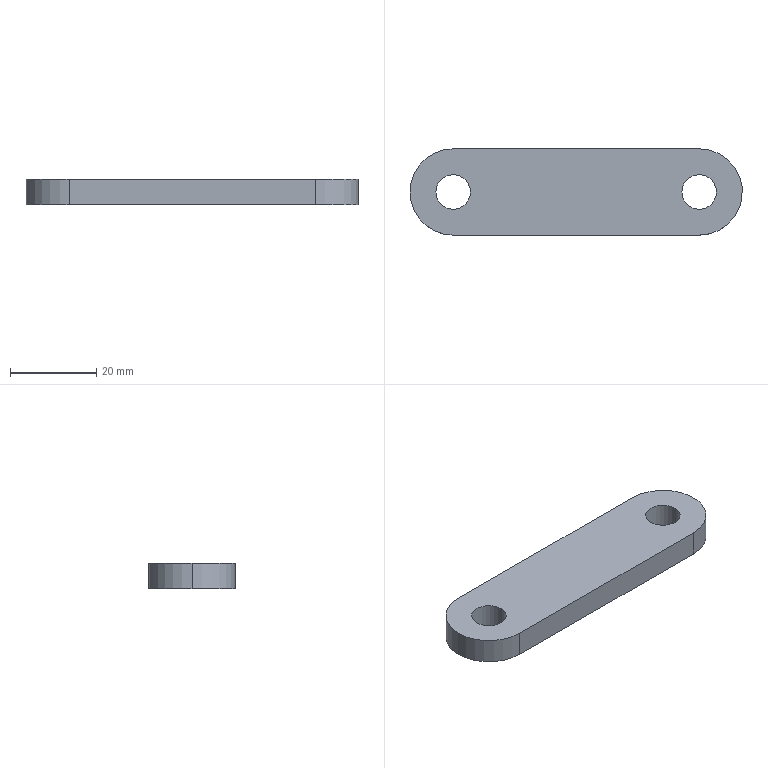Part | SolidWorks | features Extrusion 1, ICE 1 | 1 solid | 11 faces | box 77.02 x 20 x 6 mm | volume 8124 mm3 | cylinder 7 | plane 4 | commonest cylinder face diameters 8 x4 20 x3
STEP:
#1=CARTESIAN_POINT('',(53.02,0.,0.));
#2=VERTEX_POINT('',#1);
#3=CARTESIAN_POINT('',(61.02,0.,0.));
#4=VERTEX_POINT('',#3);
#5=CARTESIAN_POINT('',(57.02,0.,0.));
#6=DIRECTION('',(0.,0.,1.));
#7=DIRECTION('',(1.,0.,0.));
#8=AXIS2_PLACEMENT_3D('',#5,#6,#7);
#9=CIRCLE('',#8,4.);
#10=EDGE_CURVE('',#2,#4,#9,.T.);
#11=ORIENTED_EDGE('',*,*,#10,.F.);
#12=CARTESIAN_POINT('',(53.02,0.,6.));
#13=VERTEX_POINT('',#12);
#14=CARTESIAN_POINT('',(53.02,0.,-89.));
#15=DIRECTION('',(0.,0.,1.));
#16=VECTOR('',#15,1000.);
#17=LINE('',#14,#16);
#18=EDGE_CURVE('',#2,#13,#17,.T.);
#19=ORIENTED_EDGE('',*,*,#18,.T.);
#20=CARTESIAN_POINT('',(61.02,0.,6.));
#21=VERTEX_POINT('',#20);
#22=CARTESIAN_POINT('',(57.02,0.,6.));
#23=DIRECTION('',(0.,0.,1.));
#24=DIRECTION('',(1.,0.,0.));
#25=AXIS2_PLACEMENT_3D('',#22,#23,#24);
#26=CIRCLE('',#25,4.);
#27=EDGE_CURVE('',#13,#21,#26,.T.);
#28=ORIENTED_EDGE('',*,*,#27,.T.);
#29=CARTESIAN_POINT('',(61.02,0.,-89.));
#30=DIRECTION('',(0.,0.,1.));
#31=VECTOR('',#30,1000.);
#32=LINE('',#29,#31);
#33=EDGE_CURVE('',#4,#21,#32,.T.);
#34=ORIENTED_EDGE('',*,*,#33,.F.);
#35=EDGE_LOOP('',(#11,#19,#28,#34));
#36=FACE_OUTER_BOUND('',#35,.T.);
#37=CARTESIAN_POINT('',(57.02,0.,-89.));
#38=DIRECTION('',(0.,0.,1.));
#39=DIRECTION('',(1.,0.,0.));
#40=AXIS2_PLACEMENT_3D('',#37,#38,#39);
#41=CYLINDRICAL_SURFACE('',#40,4.);
#42=ADVANCED_FACE('',(#36),#41,.F.);
#43=CARTESIAN_POINT('',(-4.,0.,0.));
#44=VERTEX_POINT('',#43);
#45=CARTESIAN_POINT('',(4.,0.,0.));
#46=VERTEX_POINT('',#45);
#47=CARTESIAN_POINT('',(0.,0.,0.));
#48=DIRECTION('',(0.,0.,1.));
#49=DIRECTION('',(1.,0.,0.));
#50=AXIS2_PLACEMENT_3D('',#47,#48,#49);
#51=CIRCLE('',#50,4.);
#52=EDGE_CURVE('',#44,#46,#51,.T.);
#53=ORIENTED_EDGE('',*,*,#52,.F.);
#54=CARTESIAN_POINT('',(-4.,0.,6.));
#55=VERTEX_POINT('',#54);
#56=CARTESIAN_POINT('',(-4.,0.,-89.));
#57=DIRECTION('',(0.,0.,1.));
#58=VECTOR('',#57,1000.);
#59=LINE('',#56,#58);
#60=EDGE_CURVE('',#44,#55,#59,.T.);
#61=ORIENTED_EDGE('',*,*,#60,.T.);
#62=CARTESIAN_POINT('',(4.,0.,6.));
#63=VERTEX_POINT('',#62);
#64=CARTESIAN_POINT('',(0.,0.,6.));
#65=DIRECTION('',(0.,0.,1.));
#66=DIRECTION('',(1.,0.,0.));
#67=AXIS2_PLACEMENT_3D('',#64,#65,#66);
#68=CIRCLE('',#67,4.);
#69=EDGE_CURVE('',#55,#63,#68,.T.);
#70=ORIENTED_EDGE('',*,*,#69,.T.);
#71=CARTESIAN_POINT('',(4.,0.,-89.));
#72=DIRECTION('',(0.,0.,1.));
#73=VECTOR('',#72,1000.);
#74=LINE('',#71,#73);
#75=EDGE_CURVE('',#46,#63,#74,.T.);
#76=ORIENTED_EDGE('',*,*,#75,.F.);
#77=EDGE_LOOP('',(#53,#61,#70,#76));
#78=FACE_OUTER_BOUND('',#77,.T.);
#79=CARTESIAN_POINT('',(0.,0.,-89.));
#80=DIRECTION('',(0.,0.,1.));
#81=DIRECTION('',(1.,0.,0.));
#82=AXIS2_PLACEMENT_3D('',#79,#80,#81);
#83=CYLINDRICAL_SURFACE('',#82,4.);
#84=ADVANCED_FACE('',(#78),#83,.F.);
#85=CARTESIAN_POINT('',(-10.,0.,6.));
#86=VERTEX_POINT('',#85);
#87=CARTESIAN_POINT('',(0.,-10.,6.));
#88=VERTEX_POINT('',#87);
#89=CARTESIAN_POINT('',(0.,0.,6.));
#90=DIRECTION('',(0.,0.,1.));
#91=DIRECTION('',(1.,0.,0.));
#92=AXIS2_PLACEMENT_3D('',#89,#90,#91);
#93=CIRCLE('',#92,10.);
#94=EDGE_CURVE('',#86,#88,#93,.T.);
#95=ORIENTED_EDGE('',*,*,#94,.F.);
#96=CARTESIAN_POINT('',(-10.,0.,0.));
#97=VERTEX_POINT('',#96);
#98=CARTESIAN_POINT('',(-10.,0.,6.));
#99=DIRECTION('',(0.,0.,-1.));
#100=VECTOR('',#99,1000.);
#101=LINE('',#98,#100);
#102=EDGE_CURVE('',#86,#97,#101,.T.);
#103=ORIENTED_EDGE('',*,*,#102,.T.);
#104=CARTESIAN_POINT('',(0.,-10.,0.));
#105=VERTEX_POINT('',#104);
#106=CARTESIAN_POINT('',(0.,0.,0.));
#107=DIRECTION('',(0.,0.,1.));
#108=DIRECTION('',(1.,0.,0.));
#109=AXIS2_PLACEMENT_3D('',#106,#107,#108);
#110=CIRCLE('',#109,10.);
#111=EDGE_CURVE('',#97,#105,#110,.T.);
#112=ORIENTED_EDGE('',*,*,#111,.T.);
#113=CARTESIAN_POINT('',(0.,-10.,6.));
#114=DIRECTION('',(0.,0.,-1.));
#115=VECTOR('',#114,1000.);
#116=LINE('',#113,#115);
#117=EDGE_CURVE('',#88,#105,#116,.T.);
#118=ORIENTED_EDGE('',*,*,#117,.F.);
#119=EDGE_LOOP('',(#95,#103,#112,#118));
#120=FACE_OUTER_BOUND('',#119,.T.);
#121=CARTESIAN_POINT('',(0.,0.,6.));
#122=DIRECTION('',(0.,0.,-1.));
#123=DIRECTION('',(-1.,0.,0.));
#124=AXIS2_PLACEMENT_3D('',#121,#122,#123);
#125=CYLINDRICAL_SURFACE('',#124,10.);
#126=ADVANCED_FACE('',(#120),#125,.T.);
#127=ORIENTED_EDGE('',*,*,#102,.F.);
#128=CARTESIAN_POINT('',(0.,10.,6.));
#129=VERTEX_POINT('',#128);
#130=CARTESIAN_POINT('',(0.,0.,6.));
#131=DIRECTION('',(0.,0.,1.));
#132=DIRECTION('',(1.,0.,0.));
#133=AXIS2_PLACEMENT_3D('',#130,#131,#132);
#134=CIRCLE('',#133,10.);
#135=EDGE_CURVE('',#129,#86,#134,.T.);
#136=ORIENTED_EDGE('',*,*,#135,.F.);
#137=CARTESIAN_POINT('',(0.,10.,0.));
#138=VERTEX_POINT('',#137);
#139=CARTESIAN_POINT('',(0.,10.,6.));
#140=DIRECTION('',(0.,0.,-1.));
#141=VECTOR('',#140,1000.);
#142=LINE('',#139,#141);
#143=EDGE_CURVE('',#129,#138,#142,.T.);
#144=ORIENTED_EDGE('',*,*,#143,.T.);
#145=CARTESIAN_POINT('',(0.,0.,0.));
#146=DIRECTION('',(0.,0.,1.));
#147=DIRECTION('',(1.,0.,0.));
#148=AXIS2_PLACEMENT_3D('',#145,#146,#147);
#149=CIRCLE('',#148,10.);
#150=EDGE_CURVE('',#138,#97,#149,.T.);
#151=ORIENTED_EDGE('',*,*,#150,.T.);
#152=EDGE_LOOP('',(#127,#136,#144,#151));
#153=FACE_OUTER_BOUND('',#152,.T.);
#154=CARTESIAN_POINT('',(0.,0.,6.));
#155=DIRECTION('',(0.,0.,-1.));
#156=DIRECTION('',(-1.,0.,0.));
#157=AXIS2_PLACEMENT_3D('',#154,#155,#156);
#158=CYLINDRICAL_SURFACE('',#157,10.);
#159=ADVANCED_FACE('',(#153),#158,.T.);
#160=CARTESIAN_POINT('',(57.02,-10.,0.));
#161=VERTEX_POINT('',#160);
#162=CARTESIAN_POINT('',(0.,-10.,0.));
#163=DIRECTION('',(1.,0.,0.));
#164=VECTOR('',#163,1000.);
#165=LINE('',#162,#164);
#166=EDGE_CURVE('',#105,#161,#165,.T.);
#167=ORIENTED_EDGE('',*,*,#166,.T.);
#168=CARTESIAN_POINT('',(57.02,-10.,6.));
#169=VERTEX_POINT('',#168);
#170=CARTESIAN_POINT('',(57.02,-10.,6.));
#171=DIRECTION('',(0.,0.,-1.));
#172=VECTOR('',#171,1000.);
#173=LINE('',#170,#172);
#174=EDGE_CURVE('',#169,#161,#173,.T.);
#175=ORIENTED_EDGE('',*,*,#174,.F.);
#176=CARTESIAN_POINT('',(0.,-10.,6.));
#177=DIRECTION('',(1.,0.,0.));
#178=VECTOR('',#177,1000.);
#179=LINE('',#176,#178);
#180=EDGE_CURVE('',#88,#169,#179,.T.);
#181=ORIENTED_EDGE('',*,*,#180,.F.);
#182=ORIENTED_EDGE('',*,*,#117,.T.);
#183=EDGE_LOOP('',(#167,#175,#181,#182));
#184=FACE_OUTER_BOUND('',#183,.T.);
#185=CARTESIAN_POINT('',(0.,-10.,6.));
#186=DIRECTION('',(0.,1.,0.));
#187=DIRECTION('',(0.,0.,1.));
#188=AXIS2_PLACEMENT_3D('',#185,#186,#187);
#189=PLANE('',#188);
#190=ADVANCED_FACE('',(#184),#189,.F.);
#191=CARTESIAN_POINT('',(57.02,10.,0.));
#192=VERTEX_POINT('',#191);
#193=CARTESIAN_POINT('',(57.02,0.,0.));
#194=DIRECTION('',(0.,0.,1.));
#195=DIRECTION('',(1.,0.,0.));
#196=AXIS2_PLACEMENT_3D('',#193,#194,#195);
#197=CIRCLE('',#196,10.);
#198=EDGE_CURVE('',#161,#192,#197,.T.);
#199=ORIENTED_EDGE('',*,*,#198,.T.);
#200=CARTESIAN_POINT('',(57.02,10.,6.));
#201=VERTEX_POINT('',#200);
#202=CARTESIAN_POINT('',(57.02,10.,6.));
#203=DIRECTION('',(0.,0.,-1.));
#204=VECTOR('',#203,1000.);
#205=LINE('',#202,#204);
#206=EDGE_CURVE('',#201,#192,#205,.T.);
#207=ORIENTED_EDGE('',*,*,#206,.F.);
#208=CARTESIAN_POINT('',(57.02,0.,6.));
#209=DIRECTION('',(0.,0.,1.));
#210=DIRECTION('',(1.,0.,0.));
#211=AXIS2_PLACEMENT_3D('',#208,#209,#210);
#212=CIRCLE('',#211,10.);
#213=EDGE_CURVE('',#169,#201,#212,.T.);
#214=ORIENTED_EDGE('',*,*,#213,.F.);
#215=ORIENTED_EDGE('',*,*,#174,.T.);
#216=EDGE_LOOP('',(#199,#207,#214,#215));
#217=FACE_OUTER_BOUND('',#216,.T.);
#218=CARTESIAN_POINT('',(57.02,0.,6.));
#219=DIRECTION('',(0.,0.,-1.));
#220=DIRECTION('',(-1.,0.,0.));
#221=AXIS2_PLACEMENT_3D('',#218,#219,#220);
#222=CYLINDRICAL_SURFACE('',#221,10.);
#223=ADVANCED_FACE('',(#217),#222,.T.);
#224=CARTESIAN_POINT('',(0.,10.,0.));
#225=DIRECTION('',(-1.,0.,0.));
#226=VECTOR('',#225,1000.);
#227=LINE('',#224,#226);
#228=EDGE_CURVE('',#192,#138,#227,.T.);
#229=ORIENTED_EDGE('',*,*,#228,.T.);
#230=ORIENTED_EDGE('',*,*,#143,.F.);
#231=CARTESIAN_POINT('',(0.,10.,6.));
#232=DIRECTION('',(-1.,0.,0.));
#233=VECTOR('',#232,1000.);
#234=LINE('',#231,#233);
#235=EDGE_CURVE('',#201,#129,#234,.T.);
#236=ORIENTED_EDGE('',*,*,#235,.F.);
#237=ORIENTED_EDGE('',*,*,#206,.T.);
#238=EDGE_LOOP('',(#229,#230,#236,#237));
#239=FACE_OUTER_BOUND('',#238,.T.);
#240=CARTESIAN_POINT('',(0.,10.,6.));
#241=DIRECTION('',(0.,-1.,0.));
#242=DIRECTION('',(0.,0.,-1.));
#243=AXIS2_PLACEMENT_3D('',#240,#241,#242);
#244=PLANE('',#243);
#245=ADVANCED_FACE('',(#239),#244,.F.);
#246=CARTESIAN_POINT('',(57.02,0.,6.));
#247=DIRECTION('',(0.,0.,1.));
#248=DIRECTION('',(1.,0.,0.));
#249=AXIS2_PLACEMENT_3D('',#246,#247,#248);
#250=CIRCLE('',#249,4.);
#251=EDGE_CURVE('',#21,#13,#250,.T.);
#252=ORIENTED_EDGE('',*,*,#251,.F.);
#253=ORIENTED_EDGE('',*,*,#27,.F.);
#254=EDGE_LOOP('',(#252,#253));
#255=FACE_BOUND('',#254,.T.);
#256=CARTESIAN_POINT('',(0.,0.,6.));
#257=DIRECTION('',(0.,0.,1.));
#258=DIRECTION('',(1.,0.,0.));
#259=AXIS2_PLACEMENT_3D('',#256,#257,#258);
#260=CIRCLE('',#259,4.);
#261=EDGE_CURVE('',#63,#55,#260,.T.);
#262=ORIENTED_EDGE('',*,*,#261,.F.);
#263=ORIENTED_EDGE('',*,*,#69,.F.);
#264=EDGE_LOOP('',(#262,#263));
#265=FACE_BOUND('',#264,.T.);
#266=ORIENTED_EDGE('',*,*,#135,.T.);
#267=ORIENTED_EDGE('',*,*,#94,.T.);
#268=ORIENTED_EDGE('',*,*,#180,.T.);
#269=ORIENTED_EDGE('',*,*,#213,.T.);
#270=ORIENTED_EDGE('',*,*,#235,.T.);
#271=EDGE_LOOP('',(#266,#267,#268,#269,#270));
#272=FACE_OUTER_BOUND('',#271,.T.);
#273=CARTESIAN_POINT('',(0.,0.,6.));
#274=DIRECTION('',(0.,0.,1.));
#275=DIRECTION('',(1.,0.,0.));
#276=AXIS2_PLACEMENT_3D('',#273,#274,#275);
#277=PLANE('',#276);
#278=ADVANCED_FACE('',(#255,#265,#272),#277,.T.);
#279=CARTESIAN_POINT('',(57.02,0.,0.));
#280=DIRECTION('',(0.,0.,1.));
#281=DIRECTION('',(1.,0.,0.));
#282=AXIS2_PLACEMENT_3D('',#279,#280,#281);
#283=CIRCLE('',#282,4.);
#284=EDGE_CURVE('',#4,#2,#283,.T.);
#285=ORIENTED_EDGE('',*,*,#284,.T.);
#286=ORIENTED_EDGE('',*,*,#10,.T.);
#287=EDGE_LOOP('',(#285,#286));
#288=FACE_BOUND('',#287,.T.);
#289=CARTESIAN_POINT('',(0.,0.,0.));
#290=DIRECTION('',(0.,0.,1.));
#291=DIRECTION('',(1.,0.,0.));
#292=AXIS2_PLACEMENT_3D('',#289,#290,#291);
#293=CIRCLE('',#292,4.);
#294=EDGE_CURVE('',#46,#44,#293,.T.);
#295=ORIENTED_EDGE('',*,*,#294,.T.);
#296=ORIENTED_EDGE('',*,*,#52,.T.);
#297=EDGE_LOOP('',(#295,#296));
#298=FACE_BOUND('',#297,.T.);
#299=ORIENTED_EDGE('',*,*,#150,.F.);
#300=ORIENTED_EDGE('',*,*,#228,.F.);
#301=ORIENTED_EDGE('',*,*,#198,.F.);
#302=ORIENTED_EDGE('',*,*,#166,.F.);
#303=ORIENTED_EDGE('',*,*,#111,.F.);
#304=EDGE_LOOP('',(#299,#300,#301,#302,#303));
#305=FACE_OUTER_BOUND('',#304,.T.);
#306=CARTESIAN_POINT('',(0.,0.,0.));
#307=DIRECTION('',(0.,0.,1.));
#308=DIRECTION('',(1.,0.,0.));
#309=AXIS2_PLACEMENT_3D('',#306,#307,#308);
#310=PLANE('',#309);
#311=ADVANCED_FACE('',(#288,#298,#305),#310,.F.);
#312=ORIENTED_EDGE('',*,*,#60,.F.);
#313=ORIENTED_EDGE('',*,*,#294,.F.);
#314=ORIENTED_EDGE('',*,*,#75,.T.);
#315=ORIENTED_EDGE('',*,*,#261,.T.);
#316=EDGE_LOOP('',(#312,#313,#314,#315));
#317=FACE_OUTER_BOUND('',#316,.T.);
#318=CARTESIAN_POINT('',(0.,0.,-89.));
#319=DIRECTION('',(0.,0.,1.));
#320=DIRECTION('',(1.,0.,0.));
#321=AXIS2_PLACEMENT_3D('',#318,#319,#320);
#322=CYLINDRICAL_SURFACE('',#321,4.);
#323=ADVANCED_FACE('',(#317),#322,.F.);
#324=ORIENTED_EDGE('',*,*,#18,.F.);
#325=ORIENTED_EDGE('',*,*,#284,.F.);
#326=ORIENTED_EDGE('',*,*,#33,.T.);
#327=ORIENTED_EDGE('',*,*,#251,.T.);
#328=EDGE_LOOP('',(#324,#325,#326,#327));
#329=FACE_OUTER_BOUND('',#328,.T.);
#330=CARTESIAN_POINT('',(57.02,0.,-89.));
#331=DIRECTION('',(0.,0.,1.));
#332=DIRECTION('',(1.,0.,0.));
#333=AXIS2_PLACEMENT_3D('',#330,#331,#332);
#334=CYLINDRICAL_SURFACE('',#333,4.);
#335=ADVANCED_FACE('',(#329),#334,.F.);
#336=CLOSED_SHELL('',(#42,#84,#126,#159,#190,#223,#245,#278,#311,#323,#335));
#337=MANIFOLD_SOLID_BREP('',#336);
#338=CARTESIAN_POINT('',(0.,0.,0.));
#339=DIRECTION('',(0.,0.,1.));
#340=DIRECTION('',(1.,0.,0.));
#341=AXIS2_PLACEMENT_3D('',#338,#339,#340);
#342=(LENGTH_UNIT()NAMED_UNIT(*)SI_UNIT(.MILLI.,.METRE.));
#343=UNCERTAINTY_MEASURE_WITH_UNIT(LENGTH_MEASURE(0.00001),#342,'','');
#344=(NAMED_UNIT(*)PLANE_ANGLE_UNIT()SI_UNIT($,.RADIAN.));
#345=(NAMED_UNIT(*)SI_UNIT($,.STERADIAN.)SOLID_ANGLE_UNIT());
#346=(GEOMETRIC_REPRESENTATION_CONTEXT(3)GLOBAL_UNCERTAINTY_ASSIGNED_CONTEXT((#343))GLOBAL_UNIT_ASSIGNED_CONTEXT((#342,#344,#345))REPRESENTATION_CONTEXT('',''));
#347=ADVANCED_BREP_SHAPE_REPRESENTATION('',(#337,#341),#346);